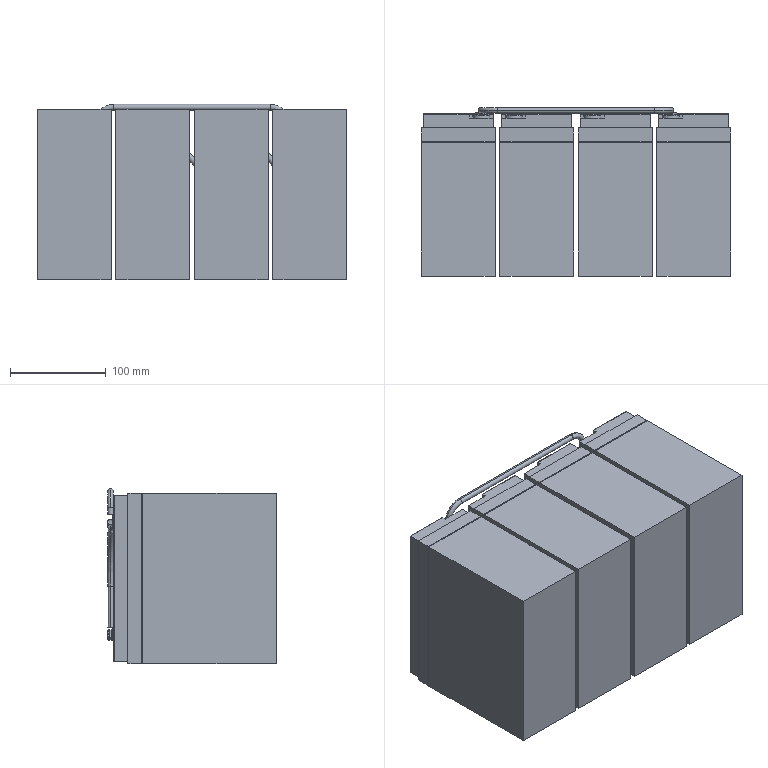Part | SolidWorks | 8 solids | 1617 faces | box 323 x 176 x 183 mm | volume 9247654 mm3 | plane 983 | spline 452 | cylinder 132 | torus 26 | cone 24 | commonest cylinder face diameters 2 x32 12 x30 6 x28 5 x16 18 x16 16 x6